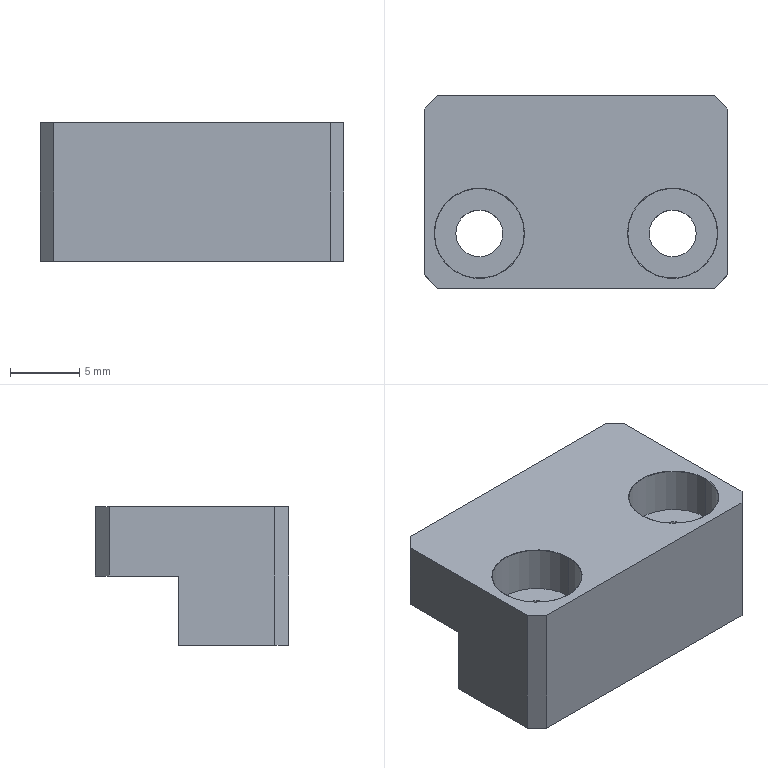Part | STEP file | QA-FB08 | 1 solid | 32 faces | box 22 x 14 x 10 mm | volume 1976 mm3 | plane 16 | cylinder 12 | cone 4 | commonest cylinder face diameters 3.4 x4 4.2 x4 6.5 x4